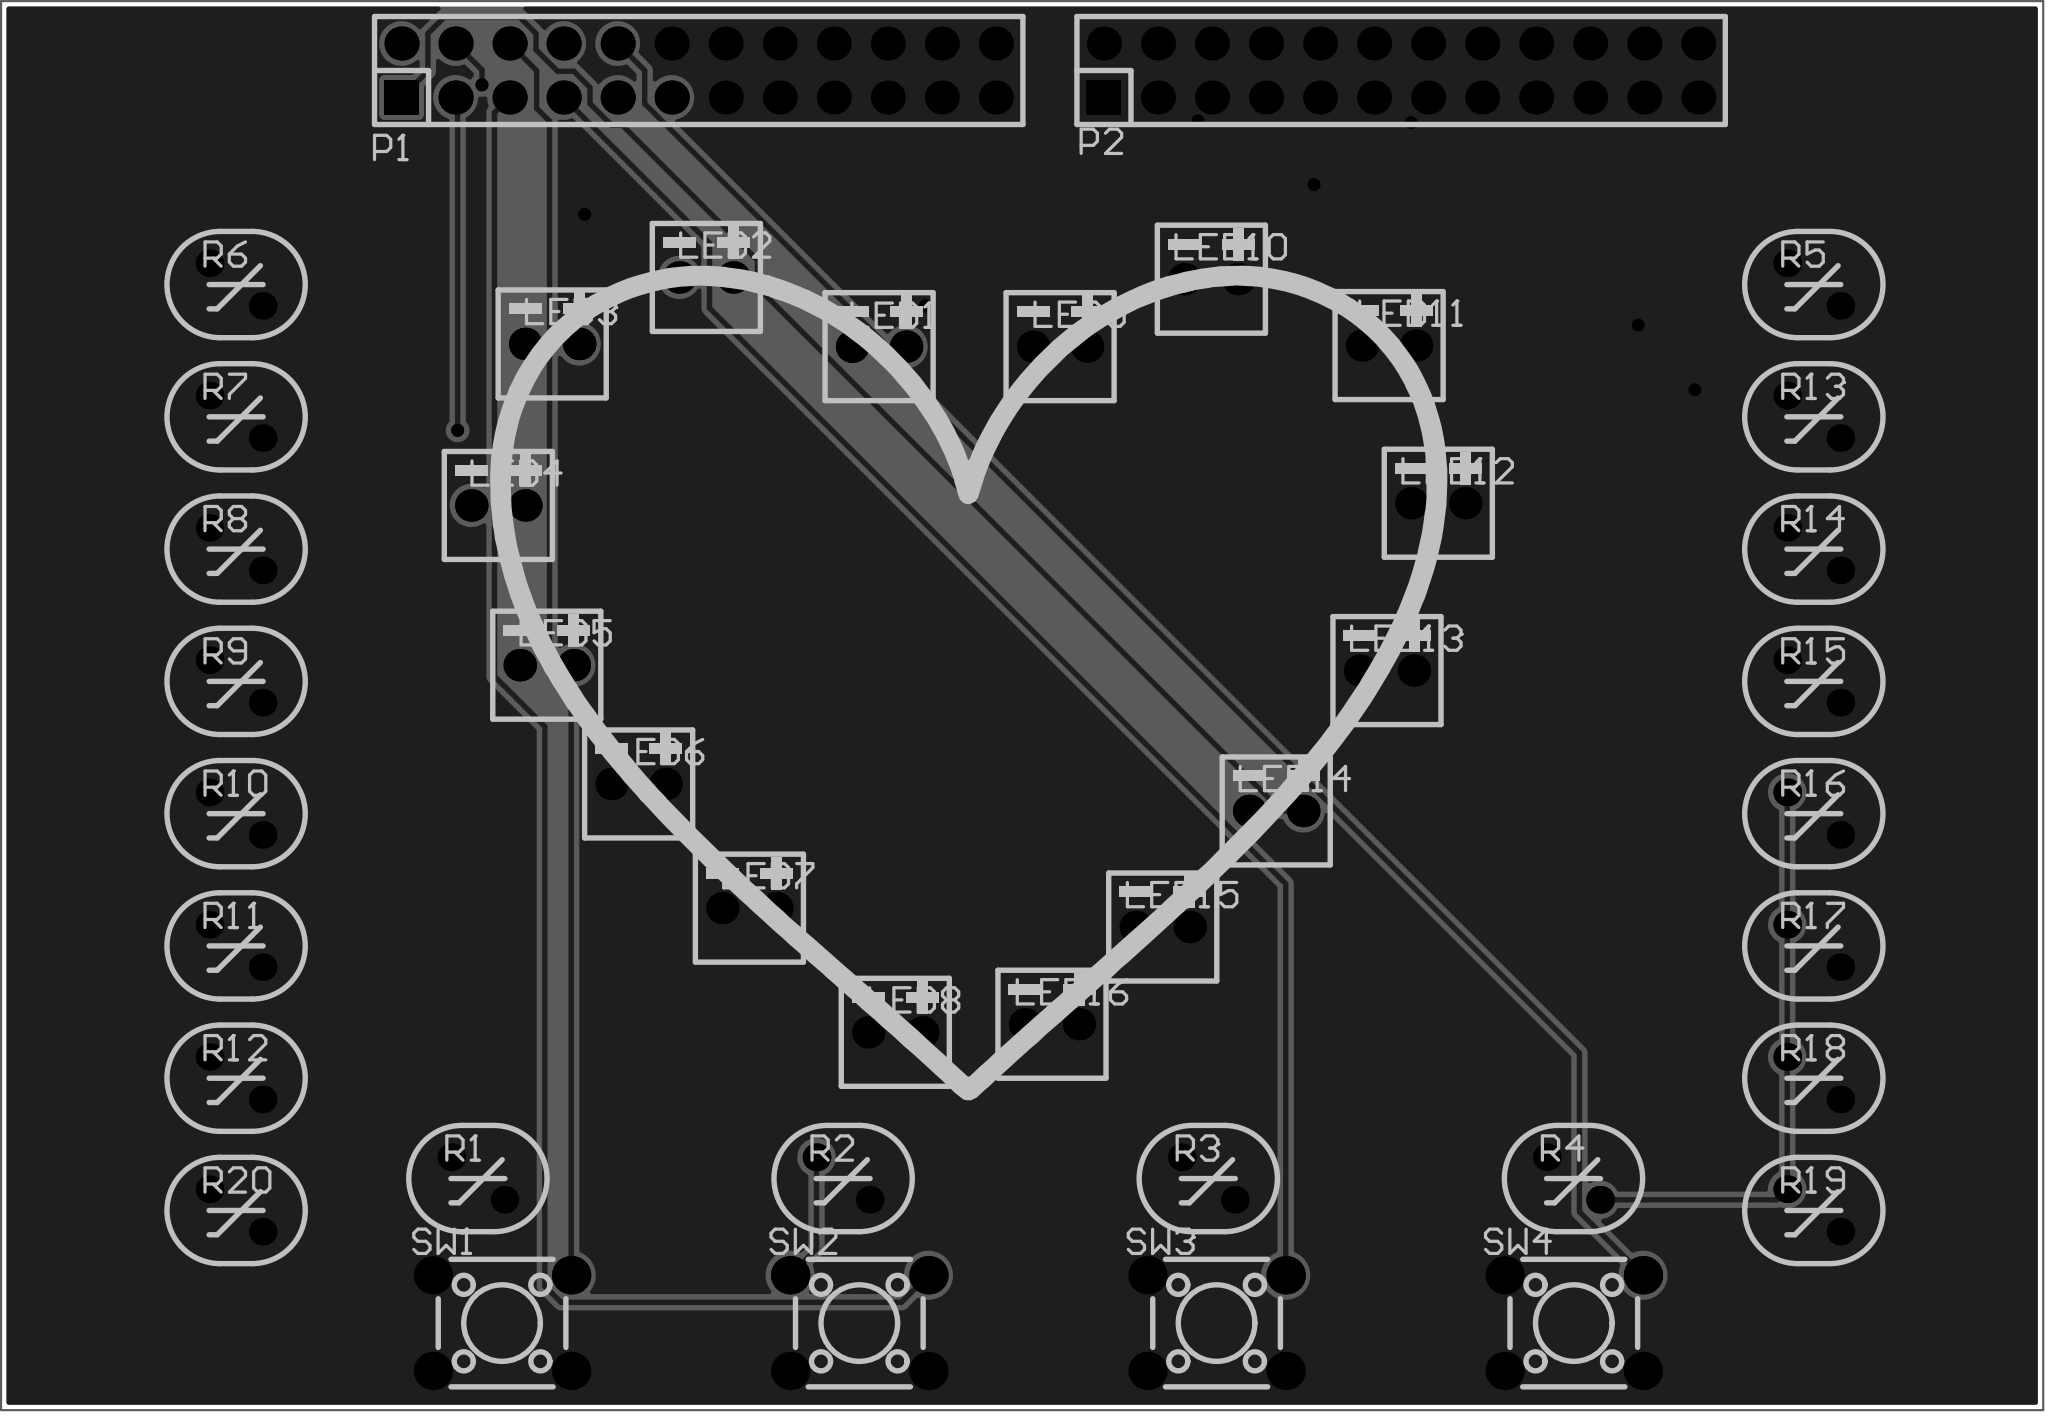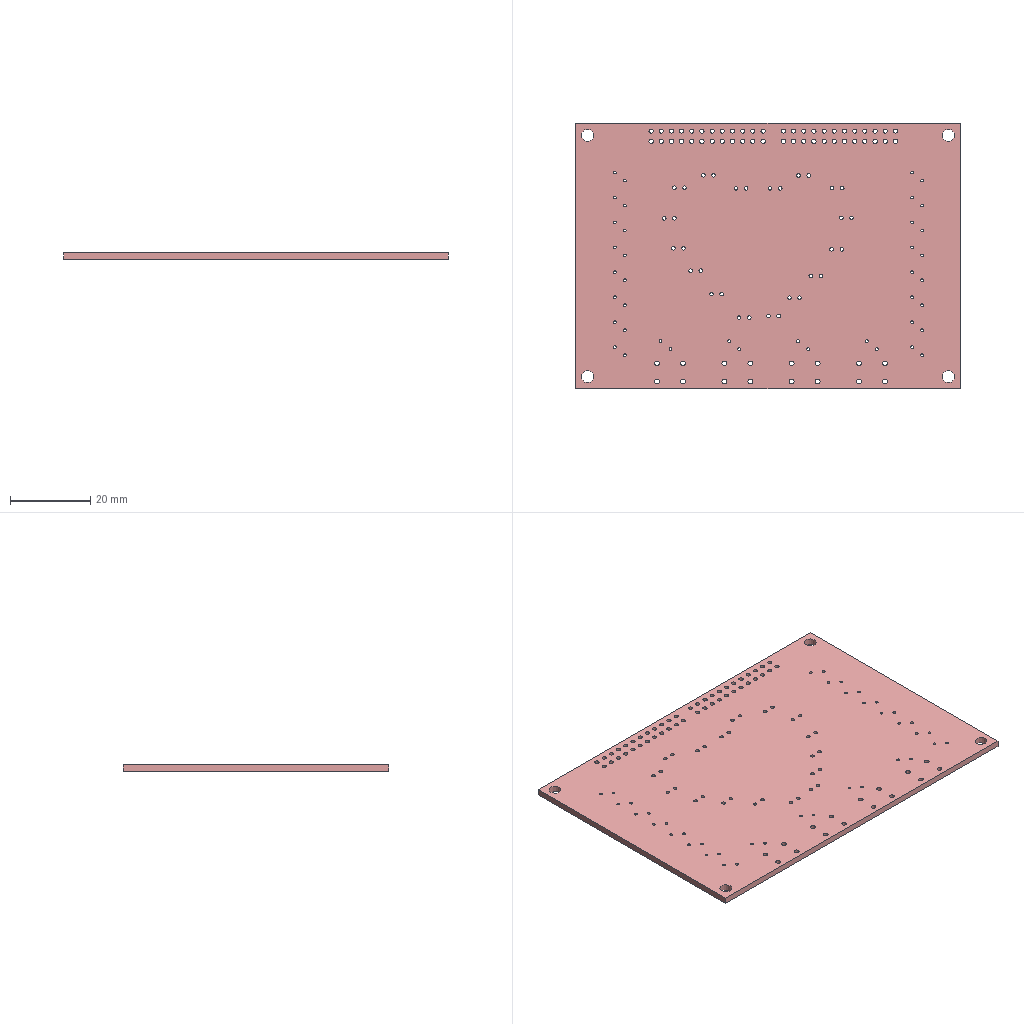Circuit board layout | Altium Designer | box 96 x 66.3 x 1.6 mm
Layer stack:
# Altium Designer layer stack of  (unit mm; dielectric type: 0 none, 1 core, 2 prepreg, 3 surface material)
index,name,kind,layer,copper_thickness_mm,dielectric_type,dielectric_thickness_mm,dielectric_material,dielectric_constant
0,Top Paste Mask Layer,other,,,,,,
1,Top Silkscreen Layer,other,,,,,,
2,Top Solder Mask Layer,dielectric,,,3,0.01,,3.3
3,Top Layer,copper,Top Layer,0.035,,,,
4,Dielectric1,dielectric,,,3,1.51,FR4,4.5
5,Bottom Layer,copper,Bottom Layer,0.035,,,,
6,Bottom Solder Mask Layer,dielectric,,,3,0.01,,3.3
7,Bottom Silkscreen Layer,other,,,,,,
8,Bottom Paste Mask Layer,other,,,,,,
# drill layer pairs: low layer,high layer
drill_pair,Top Layer,Bottom Layer
Part placement:
Designator,Comment,Layer,Footprint,Center-X(mm),Center-Y(mm),Rotation
P1,2.54-2*12P female,TopLayer,HDR-TH_24P-P2.54-V-F-R2-C12-S2.54,119.791,149.516,0
P2,2.54-2*12P female,TopLayer,HDR-TH_24P-P2.54-V-F-R2-C12-S2.54,152.811,149.516,0
SW1,TS665CJ,TopLayer,SW-TH_4P-L6.0-W6.0-P4.50-LS6.5,110.546,90.588,0
SW2,TS665CJ,TopLayer,SW-TH_4P-L6.0-W6.0-P4.50-LS6.5,127.341,90.588,0
SW3,TS665CJ,TopLayer,SW-TH_4P-L6.0-W6.0-P4.50-LS6.5,144.135,90.588,0
SW4,TS665CJ,TopLayer,SW-TH_4P-L6.0-W6.0-P4.50-LS6.5,160.929,90.588,0
LED1,,TopLayer,LED-TH_L5.0-W5.0-P2.54_RED,128.27,136.525,180
LED2,,TopLayer,LED-TH_L5.0-W5.0-P2.54_RED,120.15,139.78,180
LED3,,TopLayer,LED-TH_L5.0-W5.0-P2.54_RED,112.903,136.652,180
LED4,,TopLayer,LED-TH_L5.0-W5.0-P2.54_RED,110.371,129.054,180
LED5,,TopLayer,LED-TH_L5.0-W5.0-P2.54_RED,112.649,121.539,180
LED6,,TopLayer,LED-TH_L5.0-W5.0-P2.54_RED,116.967,115.951,180
LED7,,TopLayer,LED-TH_L5.0-W5.0-P2.54_RED,122.174,110.109,180
LED8,,TopLayer,LED-TH_L5.0-W5.0-P2.54_RED,129.032,104.267,180
LED9,,TopLayer,LED-TH_L5.0-W5.0-P2.54_RED,136.779,136.525,180
LED10,,TopLayer,LED-TH_L5.0-W5.0-P2.54_RED,143.891,139.7,180
LED11,,TopLayer,LED-TH_L5.0-W5.0-P2.54_RED,152.246,136.576,180
LED12,,TopLayer,LED-TH_L5.0-W5.0-P2.54_RED,154.559,129.159,180
LED13,,TopLayer,LED-TH_L5.0-W5.0-P2.54_RED,152.146,121.285,180
LED14,,TopLayer,LED-TH_L5.0-W5.0-P2.54_RED,146.939,114.681,180
LED15,,TopLayer,LED-TH_L5.0-W5.0-P2.54_RED,141.605,109.22,180
LED16,,TopLayer,LED-TH_L5.0-W5.0-P2.54_RED,136.398,104.648,180
R1,4.7K,TopLayer,RES-TH_RES-TH_L6.5-W5.0-P2.50-D0.4-S2.00,109.411,97.387,0
R2,4.7K,TopLayer,RES-TH_RES-TH_L6.5-W5.0-P2.50-D0.4-S2.00,126.579,97.387,0
R3,4.7K,TopLayer,RES-TH_RES-TH_L6.5-W5.0-P2.50-D0.4-S2.00,143.746,97.387,0
R4,4.7K,TopLayer,RES-TH_RES-TH_L6.5-W5.0-P2.50-D0.4-S2.00,160.914,97.387,0
R5,1K,TopLayer,RES-TH_RES-TH_L6.5-W5.0-P2.50-D0.4-S2.00,172.212,139.446,0
R6,1K,TopLayer,RES-TH_RES-TH_L6.5-W5.0-P2.50-D0.4-S2.00,98.044,139.446,0
R7,1K,TopLayer,RES-TH_RES-TH_L6.5-W5.0-P2.50-D0.4-S2.00,98.044,133.223,0
R8,1K,TopLayer,RES-TH_RES-TH_L6.5-W5.0-P2.50-D0.4-S2.00,98.044,127,0
R9,1K,TopLayer,RES-TH_RES-TH_L6.5-W5.0-P2.50-D0.4-S2.00,98.044,120.777,0
R10,1K,TopLayer,RES-TH_RES-TH_L6.5-W5.0-P2.50-D0.4-S2.00,98.044,114.554,0
R11,1K,TopLayer,RES-TH_RES-TH_L6.5-W5.0-P2.50-D0.4-S2.00,98.044,108.331,0
R12,1K,TopLayer,RES-TH_RES-TH_L6.5-W5.0-P2.50-D0.4-S2.00,98.044,102.108,0
R13,1K,TopLayer,RES-TH_RES-TH_L6.5-W5.0-P2.50-D0.4-S2.00,172.212,133.223,0
R14,1K,TopLayer,RES-TH_RES-TH_L6.5-W5.0-P2.50-D0.4-S2.00,172.212,127,0
R15,1K,TopLayer,RES-TH_RES-TH_L6.5-W5.0-P2.50-D0.4-S2.00,172.212,120.777,0
R16,1K,TopLayer,RES-TH_RES-TH_L6.5-W5.0-P2.50-D0.4-S2.00,172.212,114.554,0
R17,1K,TopLayer,RES-TH_RES-TH_L6.5-W5.0-P2.50-D0.4-S2.00,172.212,108.331,0
R18,1K,TopLayer,RES-TH_RES-TH_L6.5-W5.0-P2.50-D0.4-S2.00,172.212,102.108,0
R19,1K,TopLayer,RES-TH_RES-TH_L6.5-W5.0-P2.50-D0.4-S2.00,172.212,95.885,0
R20,1K,TopLayer,RES-TH_RES-TH_L6.5-W5.0-P2.50-D0.4-S2.00,98.044,95.885,0
Pad and via stacks:
# Altium Designer via and pad stacks of  (unit mm). Each distinct definition once, with the count of objects using it.
# via: kind,start_layer,end_layer,hole_mm,diameter_mm,mode(0 simple;1 top-mid-bottom;2 full stack),diameter_per_layer,count,example_net
# pad: kind,layer,hole_mm,hole_type(0 round;1 square;2 slot),plating,top_size,top_shape(1 round;2 rect;3 octagon;9 rounded rect),mid_size,bottom_size,mode,footprint,size_per_layer,count,example
pad,Multi-Layer,1.05,0,plated,1.6x1.6,2,1.6x1.6,1.6x1.6,0,HDR-TH_24P-P2.54-V-F-R2-C12-S2.54,,2,P1.1
pad,Multi-Layer,1.05,0,plated,1.6x1.6,1,1.6x1.6,1.6x1.6,0,HDR-TH_24P-P2.54-V-F-R2-C12-S2.54,,46,P1.2
pad,Multi-Layer,1.2,0,plated,1.8x1.8,1,1.8x1.8,1.8x1.8,0,SW-TH_4P-L6.0-W6.0-P4.50-LS6.5,,16,SW1.1
pad,Multi-Layer,0.9144,0,plated,1.524x1.524,1,1.524x1.524,1.524x1.524,0,LED-TH_L5.0-W5.0-P2.54_RED,,32,LED1.2
pad,Multi-Layer,0.7,0,plated,1.3x1.3,1,1.3x1.3,1.3x1.3,0,RES-TH_RES-TH_L6.5-W5.0-P2.50-D0.4-S2.00,,40,R1.1
via,Top Layer,Bottom Layer,0.3048,0.61,0,,9,P01
Copper pours:
name,layer,net,type(0 solid;1 hatched;2 none)
Top Layer-GND,Top Layer,GND,0
Bottom Layer-GND,Bottom Layer,GND,0